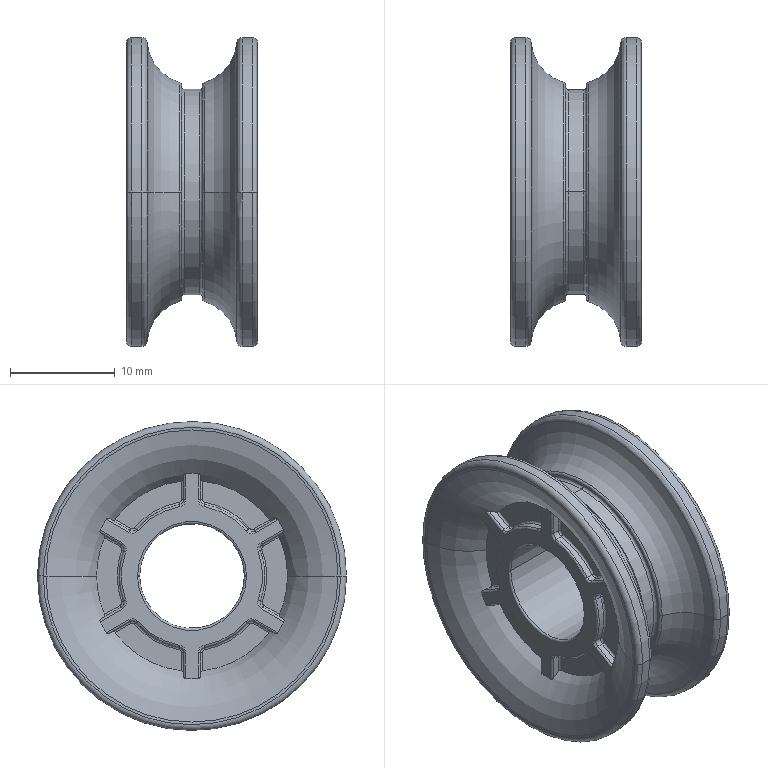Part | STEP file | MSBR-10 | 1 solid | 240 faces | box 12.49 x 29.5 x 29.5 mm | volume 3348 mm3 | cylinder 80 | torus 78 | plane 40 | spline 24 | cone 18 | commonest cylinder face diameters 0.4 x48 1 x24 29.5 x4 10 x2 19.6 x2